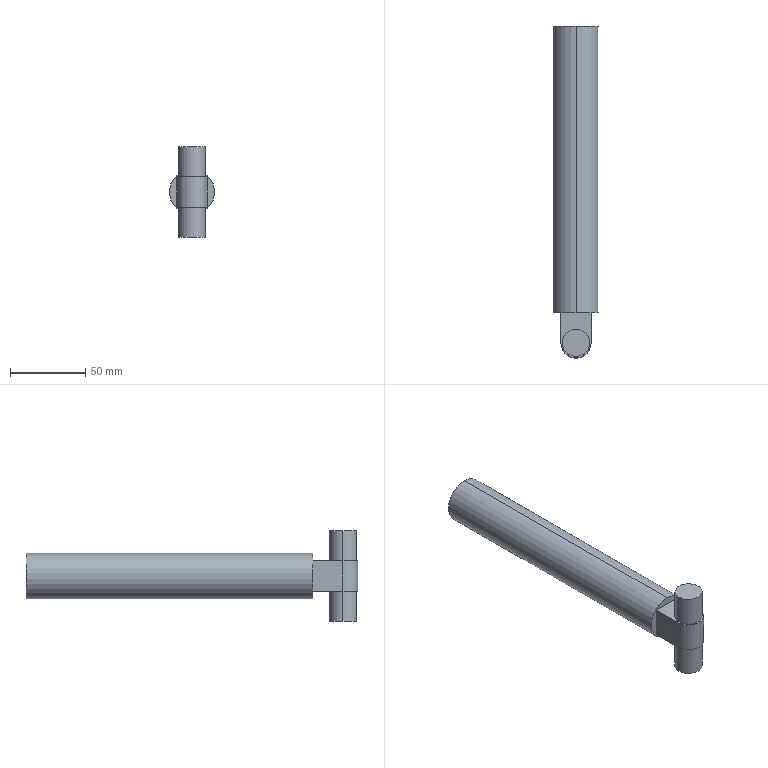Part | SolidWorks | features ICE 2, Extrusion 1 | 1 solid | 15 faces | box 30 x 220 x 60 mm | volume 155623 mm3 | plane 8 | cylinder 7 | commonest cylinder face diameters 18 x4 30 x2 20 x1
STEP:
#1=CARTESIAN_POINT('',(9.,-20.,-30.));
#2=VERTEX_POINT('',#1);
#3=CARTESIAN_POINT('',(-9.,-20.,-30.));
#4=VERTEX_POINT('',#3);
#5=CARTESIAN_POINT('',(0.,-20.,-30.));
#6=DIRECTION('',(0.,0.,1.));
#7=DIRECTION('',(1.,0.,0.));
#8=AXIS2_PLACEMENT_3D('',#5,#6,#7);
#9=CIRCLE('',#8,9.);
#10=EDGE_CURVE('',#2,#4,#9,.T.);
#11=ORIENTED_EDGE('',*,*,#10,.T.);
#12=CARTESIAN_POINT('',(-9.,-20.,-10.));
#13=VERTEX_POINT('',#12);
#14=CARTESIAN_POINT('',(-9.,-20.,-30.));
#15=DIRECTION('',(0.,0.,1.));
#16=VECTOR('',#15,1000.);
#17=LINE('',#14,#16);
#18=EDGE_CURVE('',#4,#13,#17,.T.);
#19=ORIENTED_EDGE('',*,*,#18,.T.);
#20=CARTESIAN_POINT('',(9.,-20.,-10.));
#21=VERTEX_POINT('',#20);
#22=CARTESIAN_POINT('',(0.,-20.,-10.));
#23=DIRECTION('',(0.,0.,1.));
#24=DIRECTION('',(1.,0.,0.));
#25=AXIS2_PLACEMENT_3D('',#22,#23,#24);
#26=CIRCLE('',#25,9.);
#27=EDGE_CURVE('',#21,#13,#26,.T.);
#28=ORIENTED_EDGE('',*,*,#27,.F.);
#29=CARTESIAN_POINT('',(9.,-20.,-30.));
#30=DIRECTION('',(0.,0.,1.));
#31=VECTOR('',#30,1000.);
#32=LINE('',#29,#31);
#33=EDGE_CURVE('',#2,#21,#32,.T.);
#34=ORIENTED_EDGE('',*,*,#33,.F.);
#35=EDGE_LOOP('',(#11,#19,#28,#34));
#36=FACE_OUTER_BOUND('',#35,.T.);
#37=CARTESIAN_POINT('',(0.,-20.,-30.));
#38=DIRECTION('',(0.,0.,1.));
#39=DIRECTION('',(1.,0.,0.));
#40=AXIS2_PLACEMENT_3D('',#37,#38,#39);
#41=CYLINDRICAL_SURFACE('',#40,9.);
#42=ADVANCED_FACE('',(#36),#41,.T.);
#43=CARTESIAN_POINT('',(9.,-20.,10.));
#44=VERTEX_POINT('',#43);
#45=CARTESIAN_POINT('',(-9.,-20.,10.));
#46=VERTEX_POINT('',#45);
#47=CARTESIAN_POINT('',(0.,-20.,10.));
#48=DIRECTION('',(0.,0.,1.));
#49=DIRECTION('',(1.,0.,0.));
#50=AXIS2_PLACEMENT_3D('',#47,#48,#49);
#51=CIRCLE('',#50,9.);
#52=EDGE_CURVE('',#44,#46,#51,.T.);
#53=ORIENTED_EDGE('',*,*,#52,.T.);
#54=CARTESIAN_POINT('',(-9.,-20.,30.));
#55=VERTEX_POINT('',#54);
#56=CARTESIAN_POINT('',(-9.,-20.,-30.));
#57=DIRECTION('',(0.,0.,1.));
#58=VECTOR('',#57,1000.);
#59=LINE('',#56,#58);
#60=EDGE_CURVE('',#46,#55,#59,.T.);
#61=ORIENTED_EDGE('',*,*,#60,.T.);
#62=CARTESIAN_POINT('',(9.,-20.,30.));
#63=VERTEX_POINT('',#62);
#64=CARTESIAN_POINT('',(0.,-20.,30.));
#65=DIRECTION('',(0.,0.,1.));
#66=DIRECTION('',(1.,0.,0.));
#67=AXIS2_PLACEMENT_3D('',#64,#65,#66);
#68=CIRCLE('',#67,9.);
#69=EDGE_CURVE('',#63,#55,#68,.T.);
#70=ORIENTED_EDGE('',*,*,#69,.F.);
#71=CARTESIAN_POINT('',(9.,-20.,-30.));
#72=DIRECTION('',(0.,0.,1.));
#73=VECTOR('',#72,1000.);
#74=LINE('',#71,#73);
#75=EDGE_CURVE('',#44,#63,#74,.T.);
#76=ORIENTED_EDGE('',*,*,#75,.F.);
#77=EDGE_LOOP('',(#53,#61,#70,#76));
#78=FACE_OUTER_BOUND('',#77,.T.);
#79=CARTESIAN_POINT('',(0.,-20.,-30.));
#80=DIRECTION('',(0.,0.,1.));
#81=DIRECTION('',(1.,0.,0.));
#82=AXIS2_PLACEMENT_3D('',#79,#80,#81);
#83=CYLINDRICAL_SURFACE('',#82,9.);
#84=ADVANCED_FACE('',(#78),#83,.T.);
#85=CARTESIAN_POINT('',(0.,190.,15.));
#86=VERTEX_POINT('',#85);
#87=CARTESIAN_POINT('',(0.,190.,-15.));
#88=VERTEX_POINT('',#87);
#89=CARTESIAN_POINT('',(0.,190.,0.));
#90=DIRECTION('',(0.,1.,0.));
#91=DIRECTION('',(0.,0.,1.));
#92=AXIS2_PLACEMENT_3D('',#89,#90,#91);
#93=CIRCLE('',#92,15.);
#94=EDGE_CURVE('',#86,#88,#93,.T.);
#95=ORIENTED_EDGE('',*,*,#94,.F.);
#96=CARTESIAN_POINT('',(0.,0.,15.));
#97=VERTEX_POINT('',#96);
#98=CARTESIAN_POINT('',(0.,190.,15.));
#99=DIRECTION('',(0.,-1.,0.));
#100=VECTOR('',#99,1000.);
#101=LINE('',#98,#100);
#102=EDGE_CURVE('',#86,#97,#101,.T.);
#103=ORIENTED_EDGE('',*,*,#102,.T.);
#104=CARTESIAN_POINT('',(0.,0.,-15.));
#105=VERTEX_POINT('',#104);
#106=CARTESIAN_POINT('',(0.,0.,0.));
#107=DIRECTION('',(0.,1.,0.));
#108=DIRECTION('',(0.,0.,1.));
#109=AXIS2_PLACEMENT_3D('',#106,#107,#108);
#110=CIRCLE('',#109,15.);
#111=EDGE_CURVE('',#97,#105,#110,.T.);
#112=ORIENTED_EDGE('',*,*,#111,.T.);
#113=CARTESIAN_POINT('',(0.,190.,-15.));
#114=DIRECTION('',(0.,-1.,0.));
#115=VECTOR('',#114,1000.);
#116=LINE('',#113,#115);
#117=EDGE_CURVE('',#88,#105,#116,.T.);
#118=ORIENTED_EDGE('',*,*,#117,.F.);
#119=EDGE_LOOP('',(#95,#103,#112,#118));
#120=FACE_OUTER_BOUND('',#119,.T.);
#121=CARTESIAN_POINT('',(0.,190.,0.));
#122=DIRECTION('',(0.,-1.,0.));
#123=DIRECTION('',(0.,0.,-1.));
#124=AXIS2_PLACEMENT_3D('',#121,#122,#123);
#125=CYLINDRICAL_SURFACE('',#124,15.);
#126=ADVANCED_FACE('',(#120),#125,.T.);
#127=CARTESIAN_POINT('',(0.,0.,0.));
#128=DIRECTION('',(0.,1.,0.));
#129=DIRECTION('',(0.,0.,1.));
#130=AXIS2_PLACEMENT_3D('',#127,#128,#129);
#131=CIRCLE('',#130,15.);
#132=EDGE_CURVE('',#105,#97,#131,.T.);
#133=ORIENTED_EDGE('',*,*,#132,.F.);
#134=ORIENTED_EDGE('',*,*,#111,.F.);
#135=EDGE_LOOP('',(#133,#134));
#136=FACE_OUTER_BOUND('',#135,.T.);
#137=CARTESIAN_POINT('',(-10.,0.,-10.));
#138=VERTEX_POINT('',#137);
#139=CARTESIAN_POINT('',(10.,0.,-10.));
#140=VERTEX_POINT('',#139);
#141=CARTESIAN_POINT('',(0.,0.,-10.));
#142=DIRECTION('',(1.,0.,0.));
#143=VECTOR('',#142,1000.);
#144=LINE('',#141,#143);
#145=EDGE_CURVE('',#138,#140,#144,.T.);
#146=ORIENTED_EDGE('',*,*,#145,.F.);
#147=CARTESIAN_POINT('',(-10.,0.,10.));
#148=VERTEX_POINT('',#147);
#149=CARTESIAN_POINT('',(-10.,0.,-10.));
#150=DIRECTION('',(0.,0.,1.));
#151=VECTOR('',#150,1000.);
#152=LINE('',#149,#151);
#153=EDGE_CURVE('',#138,#148,#152,.T.);
#154=ORIENTED_EDGE('',*,*,#153,.T.);
#155=CARTESIAN_POINT('',(10.,0.,10.));
#156=VERTEX_POINT('',#155);
#157=CARTESIAN_POINT('',(0.,0.,10.));
#158=DIRECTION('',(1.,0.,0.));
#159=VECTOR('',#158,1000.);
#160=LINE('',#157,#159);
#161=EDGE_CURVE('',#148,#156,#160,.T.);
#162=ORIENTED_EDGE('',*,*,#161,.T.);
#163=CARTESIAN_POINT('',(10.,0.,-10.));
#164=DIRECTION('',(0.,0.,1.));
#165=VECTOR('',#164,1000.);
#166=LINE('',#163,#165);
#167=EDGE_CURVE('',#140,#156,#166,.T.);
#168=ORIENTED_EDGE('',*,*,#167,.F.);
#169=EDGE_LOOP('',(#146,#154,#162,#168));
#170=FACE_BOUND('',#169,.T.);
#171=CARTESIAN_POINT('',(0.,0.,0.));
#172=DIRECTION('',(0.,1.,0.));
#173=DIRECTION('',(0.,0.,1.));
#174=AXIS2_PLACEMENT_3D('',#171,#172,#173);
#175=PLANE('',#174);
#176=ADVANCED_FACE('',(#136,#170),#175,.F.);
#177=ORIENTED_EDGE('',*,*,#102,.F.);
#178=CARTESIAN_POINT('',(0.,190.,0.));
#179=DIRECTION('',(0.,1.,0.));
#180=DIRECTION('',(0.,0.,1.));
#181=AXIS2_PLACEMENT_3D('',#178,#179,#180);
#182=CIRCLE('',#181,15.);
#183=EDGE_CURVE('',#88,#86,#182,.T.);
#184=ORIENTED_EDGE('',*,*,#183,.F.);
#185=ORIENTED_EDGE('',*,*,#117,.T.);
#186=ORIENTED_EDGE('',*,*,#132,.T.);
#187=EDGE_LOOP('',(#177,#184,#185,#186));
#188=FACE_OUTER_BOUND('',#187,.T.);
#189=CARTESIAN_POINT('',(0.,190.,0.));
#190=DIRECTION('',(0.,-1.,0.));
#191=DIRECTION('',(0.,0.,-1.));
#192=AXIS2_PLACEMENT_3D('',#189,#190,#191);
#193=CYLINDRICAL_SURFACE('',#192,15.);
#194=ADVANCED_FACE('',(#188),#193,.T.);
#195=ORIENTED_EDGE('',*,*,#183,.T.);
#196=ORIENTED_EDGE('',*,*,#94,.T.);
#197=EDGE_LOOP('',(#195,#196));
#198=FACE_OUTER_BOUND('',#197,.T.);
#199=CARTESIAN_POINT('',(0.,190.,0.));
#200=DIRECTION('',(0.,1.,0.));
#201=DIRECTION('',(0.,0.,1.));
#202=AXIS2_PLACEMENT_3D('',#199,#200,#201);
#203=PLANE('',#202);
#204=ADVANCED_FACE('',(#198),#203,.T.);
#205=ORIENTED_EDGE('',*,*,#27,.T.);
#206=CARTESIAN_POINT('',(0.,-20.,-10.));
#207=DIRECTION('',(0.,0.,1.));
#208=DIRECTION('',(1.,0.,0.));
#209=AXIS2_PLACEMENT_3D('',#206,#207,#208);
#210=CIRCLE('',#209,9.);
#211=EDGE_CURVE('',#13,#21,#210,.T.);
#212=ORIENTED_EDGE('',*,*,#211,.T.);
#213=EDGE_LOOP('',(#205,#212));
#214=FACE_BOUND('',#213,.T.);
#215=CARTESIAN_POINT('',(-10.,-20.,-10.));
#216=VERTEX_POINT('',#215);
#217=CARTESIAN_POINT('',(-10.,0.,-10.));
#218=DIRECTION('',(0.,-1.,0.));
#219=VECTOR('',#218,1000.);
#220=LINE('',#217,#219);
#221=EDGE_CURVE('',#138,#216,#220,.T.);
#222=ORIENTED_EDGE('',*,*,#221,.F.);
#223=ORIENTED_EDGE('',*,*,#145,.T.);
#224=CARTESIAN_POINT('',(10.,-20.,-10.));
#225=VERTEX_POINT('',#224);
#226=CARTESIAN_POINT('',(10.,0.,-10.));
#227=DIRECTION('',(0.,1.,0.));
#228=VECTOR('',#227,1000.);
#229=LINE('',#226,#228);
#230=EDGE_CURVE('',#225,#140,#229,.T.);
#231=ORIENTED_EDGE('',*,*,#230,.F.);
#232=CARTESIAN_POINT('',(0.,-20.,-10.));
#233=DIRECTION('',(0.,0.,1.));
#234=DIRECTION('',(1.,0.,0.));
#235=AXIS2_PLACEMENT_3D('',#232,#233,#234);
#236=CIRCLE('',#235,10.);
#237=EDGE_CURVE('',#216,#225,#236,.T.);
#238=ORIENTED_EDGE('',*,*,#237,.F.);
#239=EDGE_LOOP('',(#222,#223,#231,#238));
#240=FACE_OUTER_BOUND('',#239,.T.);
#241=CARTESIAN_POINT('',(0.,0.,-10.));
#242=DIRECTION('',(0.,0.,1.));
#243=DIRECTION('',(1.,0.,0.));
#244=AXIS2_PLACEMENT_3D('',#241,#242,#243);
#245=PLANE('',#244);
#246=ADVANCED_FACE('',(#214,#240),#245,.F.);
#247=ORIENTED_EDGE('',*,*,#52,.F.);
#248=CARTESIAN_POINT('',(0.,-20.,10.));
#249=DIRECTION('',(0.,0.,1.));
#250=DIRECTION('',(1.,0.,0.));
#251=AXIS2_PLACEMENT_3D('',#248,#249,#250);
#252=CIRCLE('',#251,9.);
#253=EDGE_CURVE('',#46,#44,#252,.T.);
#254=ORIENTED_EDGE('',*,*,#253,.F.);
#255=EDGE_LOOP('',(#247,#254));
#256=FACE_BOUND('',#255,.T.);
#257=ORIENTED_EDGE('',*,*,#161,.F.);
#258=CARTESIAN_POINT('',(-10.,-20.,10.));
#259=VERTEX_POINT('',#258);
#260=CARTESIAN_POINT('',(-10.,0.,10.));
#261=DIRECTION('',(0.,-1.,0.));
#262=VECTOR('',#261,1000.);
#263=LINE('',#260,#262);
#264=EDGE_CURVE('',#148,#259,#263,.T.);
#265=ORIENTED_EDGE('',*,*,#264,.T.);
#266=CARTESIAN_POINT('',(10.,-20.,10.));
#267=VERTEX_POINT('',#266);
#268=CARTESIAN_POINT('',(0.,-20.,10.));
#269=DIRECTION('',(0.,0.,1.));
#270=DIRECTION('',(1.,0.,0.));
#271=AXIS2_PLACEMENT_3D('',#268,#269,#270);
#272=CIRCLE('',#271,10.);
#273=EDGE_CURVE('',#259,#267,#272,.T.);
#274=ORIENTED_EDGE('',*,*,#273,.T.);
#275=CARTESIAN_POINT('',(10.,0.,10.));
#276=DIRECTION('',(0.,1.,0.));
#277=VECTOR('',#276,1000.);
#278=LINE('',#275,#277);
#279=EDGE_CURVE('',#267,#156,#278,.T.);
#280=ORIENTED_EDGE('',*,*,#279,.T.);
#281=EDGE_LOOP('',(#257,#265,#274,#280));
#282=FACE_OUTER_BOUND('',#281,.T.);
#283=CARTESIAN_POINT('',(0.,0.,10.));
#284=DIRECTION('',(0.,0.,1.));
#285=DIRECTION('',(1.,0.,0.));
#286=AXIS2_PLACEMENT_3D('',#283,#284,#285);
#287=PLANE('',#286);
#288=ADVANCED_FACE('',(#256,#282),#287,.T.);
#289=ORIENTED_EDGE('',*,*,#167,.T.);
#290=ORIENTED_EDGE('',*,*,#279,.F.);
#291=CARTESIAN_POINT('',(10.,-20.,-10.));
#292=DIRECTION('',(0.,0.,1.));
#293=VECTOR('',#292,1000.);
#294=LINE('',#291,#293);
#295=EDGE_CURVE('',#225,#267,#294,.T.);
#296=ORIENTED_EDGE('',*,*,#295,.F.);
#297=ORIENTED_EDGE('',*,*,#230,.T.);
#298=EDGE_LOOP('',(#289,#290,#296,#297));
#299=FACE_OUTER_BOUND('',#298,.T.);
#300=CARTESIAN_POINT('',(10.,0.,-10.));
#301=DIRECTION('',(1.,0.,0.));
#302=DIRECTION('',(0.,1.,0.));
#303=AXIS2_PLACEMENT_3D('',#300,#301,#302);
#304=PLANE('',#303);
#305=ADVANCED_FACE('',(#299),#304,.T.);
#306=ORIENTED_EDGE('',*,*,#295,.T.);
#307=ORIENTED_EDGE('',*,*,#273,.F.);
#308=CARTESIAN_POINT('',(-10.,-20.,-10.));
#309=DIRECTION('',(0.,0.,1.));
#310=VECTOR('',#309,1000.);
#311=LINE('',#308,#310);
#312=EDGE_CURVE('',#216,#259,#311,.T.);
#313=ORIENTED_EDGE('',*,*,#312,.F.);
#314=ORIENTED_EDGE('',*,*,#237,.T.);
#315=EDGE_LOOP('',(#306,#307,#313,#314));
#316=FACE_OUTER_BOUND('',#315,.T.);
#317=CARTESIAN_POINT('',(0.,-20.,-10.));
#318=DIRECTION('',(0.,0.,1.));
#319=DIRECTION('',(1.,0.,0.));
#320=AXIS2_PLACEMENT_3D('',#317,#318,#319);
#321=CYLINDRICAL_SURFACE('',#320,10.);
#322=ADVANCED_FACE('',(#316),#321,.T.);
#323=ORIENTED_EDGE('',*,*,#312,.T.);
#324=ORIENTED_EDGE('',*,*,#264,.F.);
#325=ORIENTED_EDGE('',*,*,#153,.F.);
#326=ORIENTED_EDGE('',*,*,#221,.T.);
#327=EDGE_LOOP('',(#323,#324,#325,#326));
#328=FACE_OUTER_BOUND('',#327,.T.);
#329=CARTESIAN_POINT('',(-10.,0.,-10.));
#330=DIRECTION('',(-1.,0.,0.));
#331=DIRECTION('',(0.,0.,1.));
#332=AXIS2_PLACEMENT_3D('',#329,#330,#331);
#333=PLANE('',#332);
#334=ADVANCED_FACE('',(#328),#333,.T.);
#335=ORIENTED_EDGE('',*,*,#69,.T.);
#336=CARTESIAN_POINT('',(0.,-20.,30.));
#337=DIRECTION('',(0.,0.,1.));
#338=DIRECTION('',(1.,0.,0.));
#339=AXIS2_PLACEMENT_3D('',#336,#337,#338);
#340=CIRCLE('',#339,9.);
#341=EDGE_CURVE('',#55,#63,#340,.T.);
#342=ORIENTED_EDGE('',*,*,#341,.T.);
#343=EDGE_LOOP('',(#335,#342));
#344=FACE_OUTER_BOUND('',#343,.T.);
#345=CARTESIAN_POINT('',(0.,-20.,30.));
#346=DIRECTION('',(0.,0.,1.));
#347=DIRECTION('',(1.,0.,0.));
#348=AXIS2_PLACEMENT_3D('',#345,#346,#347);
#349=PLANE('',#348);
#350=ADVANCED_FACE('',(#344),#349,.T.);
#351=ORIENTED_EDGE('',*,*,#60,.F.);
#352=ORIENTED_EDGE('',*,*,#253,.T.);
#353=ORIENTED_EDGE('',*,*,#75,.T.);
#354=ORIENTED_EDGE('',*,*,#341,.F.);
#355=EDGE_LOOP('',(#351,#352,#353,#354));
#356=FACE_OUTER_BOUND('',#355,.T.);
#357=CARTESIAN_POINT('',(0.,-20.,-30.));
#358=DIRECTION('',(0.,0.,1.));
#359=DIRECTION('',(1.,0.,0.));
#360=AXIS2_PLACEMENT_3D('',#357,#358,#359);
#361=CYLINDRICAL_SURFACE('',#360,9.);
#362=ADVANCED_FACE('',(#356),#361,.T.);
#363=ORIENTED_EDGE('',*,*,#18,.F.);
#364=CARTESIAN_POINT('',(0.,-20.,-30.));
#365=DIRECTION('',(0.,0.,1.));
#366=DIRECTION('',(1.,0.,0.));
#367=AXIS2_PLACEMENT_3D('',#364,#365,#366);
#368=CIRCLE('',#367,9.);
#369=EDGE_CURVE('',#4,#2,#368,.T.);
#370=ORIENTED_EDGE('',*,*,#369,.T.);
#371=ORIENTED_EDGE('',*,*,#33,.T.);
#372=ORIENTED_EDGE('',*,*,#211,.F.);
#373=EDGE_LOOP('',(#363,#370,#371,#372));
#374=FACE_OUTER_BOUND('',#373,.T.);
#375=CARTESIAN_POINT('',(0.,-20.,-30.));
#376=DIRECTION('',(0.,0.,1.));
#377=DIRECTION('',(1.,0.,0.));
#378=AXIS2_PLACEMENT_3D('',#375,#376,#377);
#379=CYLINDRICAL_SURFACE('',#378,9.);
#380=ADVANCED_FACE('',(#374),#379,.T.);
#381=ORIENTED_EDGE('',*,*,#10,.F.);
#382=ORIENTED_EDGE('',*,*,#369,.F.);
#383=EDGE_LOOP('',(#381,#382));
#384=FACE_OUTER_BOUND('',#383,.T.);
#385=CARTESIAN_POINT('',(0.,-20.,-30.));
#386=DIRECTION('',(0.,0.,1.));
#387=DIRECTION('',(1.,0.,0.));
#388=AXIS2_PLACEMENT_3D('',#385,#386,#387);
#389=PLANE('',#388);
#390=ADVANCED_FACE('',(#384),#389,.F.);
#391=CLOSED_SHELL('',(#42,#84,#126,#176,#194,#204,#246,#288,#305,#322,#334,#350,#362,#380,#390));
#392=MANIFOLD_SOLID_BREP('',#391);
#393=CARTESIAN_POINT('',(0.,0.,0.));
#394=DIRECTION('',(0.,0.,1.));
#395=DIRECTION('',(1.,0.,0.));
#396=AXIS2_PLACEMENT_3D('',#393,#394,#395);
#397=(LENGTH_UNIT()NAMED_UNIT(*)SI_UNIT(.MILLI.,.METRE.));
#398=UNCERTAINTY_MEASURE_WITH_UNIT(LENGTH_MEASURE(0.00001),#397,'','');
#399=(NAMED_UNIT(*)PLANE_ANGLE_UNIT()SI_UNIT($,.RADIAN.));
#400=(NAMED_UNIT(*)SI_UNIT($,.STERADIAN.)SOLID_ANGLE_UNIT());
#401=(GEOMETRIC_REPRESENTATION_CONTEXT(3)GLOBAL_UNCERTAINTY_ASSIGNED_CONTEXT((#398))GLOBAL_UNIT_ASSIGNED_CONTEXT((#397,#399,#400))REPRESENTATION_CONTEXT('',''));
#402=ADVANCED_BREP_SHAPE_REPRESENTATION('',(#392,#396),#401);